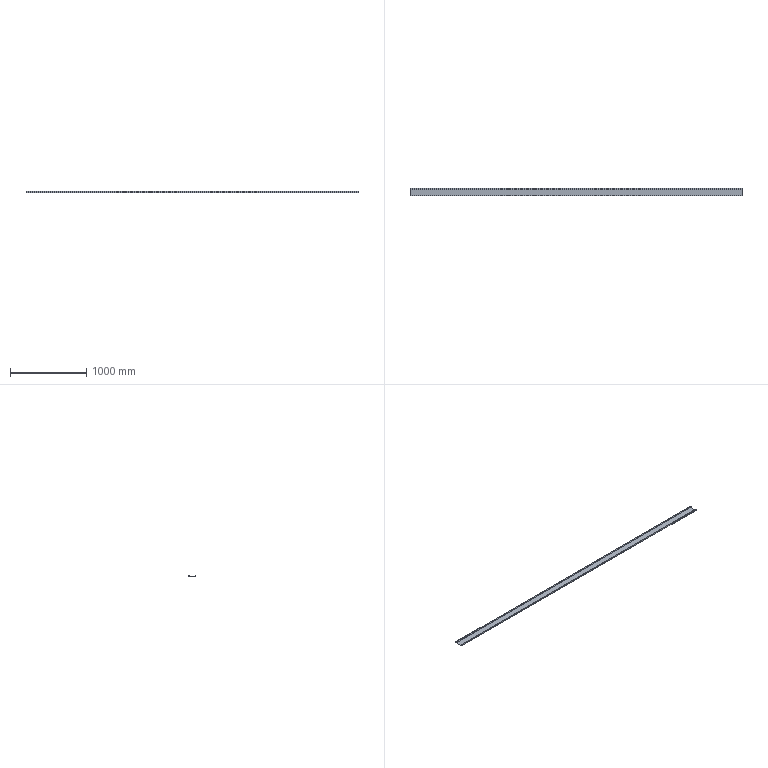Part | STEP file | 粉仓踢脚Plate 1 | 1 solid | 18 faces | box 4345 x 100 x 20 mm | volume 998785 mm3 | plane 12 | cylinder 6 | commonest cylinder face diameters 2 x3 5 x3
STEP:
#1=CARTESIAN_POINT('',(0.,0.,0.));
#2=DIRECTION('',(0.,0.,1.));
#3=DIRECTION('',(1.,0.,0.));
#4=AXIS2_PLACEMENT_3D('',#1,#2,#3);
#5=CARTESIAN_POINT('',(-2172.5,1.5,2.5));
#6=VERTEX_POINT('',#5);
#7=CARTESIAN_POINT('',(-2172.5,1.5,20.));
#8=VERTEX_POINT('',#7);
#9=CARTESIAN_POINT('',(-2172.5,1.5,2.5));
#10=DIRECTION('',(0.,0.,1.));
#11=VECTOR('',#10,1.);
#12=LINE('',#9,#11);
#13=CARTESIAN_POINT('',(2172.5,1.5,2.5));
#14=DIRECTION('',(0.,-1.,0.));
#15=DIRECTION('',(0.,0.,-1.));
#16=AXIS2_PLACEMENT_3D('',#13,#14,#15);
#17=PLANE('',#16);
#18=CARTESIAN_POINT('',(0.,-4345.));
#19=DIRECTION('',(-1.,0.));
#20=VECTOR('',#19,1.);
#21=LINE('',#18,#20);
#22=(GEOMETRIC_REPRESENTATION_CONTEXT(2)PARAMETRIC_REPRESENTATION_CONTEXT()REPRESENTATION_CONTEXT('',''));
#23=DEFINITIONAL_REPRESENTATION('',(#21),#22);
#24=PCURVE('',#17,#23);
#25=CARTESIAN_POINT('',(-2172.5,2.5,2.5));
#26=DIRECTION('',(-1.,0.,0.));
#27=DIRECTION('',(0.,0.,1.));
#28=AXIS2_PLACEMENT_3D('',#25,#26,#27);
#29=PLANE('',#28);
#30=CARTESIAN_POINT('',(0.,-1.));
#31=DIRECTION('',(1.,0.));
#32=VECTOR('',#31,1.);
#33=LINE('',#30,#32);
#34=(GEOMETRIC_REPRESENTATION_CONTEXT(2)PARAMETRIC_REPRESENTATION_CONTEXT()REPRESENTATION_CONTEXT('',''));
#35=DEFINITIONAL_REPRESENTATION('',(#33),#34);
#36=PCURVE('',#29,#35);
#37=SURFACE_CURVE('',#12,(#24,#36),.PCURVE_S1.);
#38=EDGE_CURVE('',#6,#8,#37,.T.);
#39=ORIENTED_EDGE('',*,*,#38,.T.);
#40=CARTESIAN_POINT('',(2172.5,1.5,20.));
#41=VERTEX_POINT('',#40);
#42=CARTESIAN_POINT('',(2172.5,1.5,20.));
#43=DIRECTION('',(-1.,0.,0.));
#44=VECTOR('',#43,1.);
#45=LINE('',#42,#44);
#46=CARTESIAN_POINT('',(-17.5,0.));
#47=DIRECTION('',(0.,-1.));
#48=VECTOR('',#47,1.);
#49=LINE('',#46,#48);
#50=(GEOMETRIC_REPRESENTATION_CONTEXT(2)PARAMETRIC_REPRESENTATION_CONTEXT()REPRESENTATION_CONTEXT('',''));
#51=DEFINITIONAL_REPRESENTATION('',(#49),#50);
#52=PCURVE('',#17,#51);
#53=CARTESIAN_POINT('',(2172.5,0.,20.));
#54=DIRECTION('',(0.,0.,1.));
#55=DIRECTION('',(1.,0.,0.));
#56=AXIS2_PLACEMENT_3D('',#53,#54,#55);
#57=PLANE('',#56);
#58=CARTESIAN_POINT('',(0.,1.5));
#59=DIRECTION('',(-1.,0.));
#60=VECTOR('',#59,1.);
#61=LINE('',#58,#60);
#62=(GEOMETRIC_REPRESENTATION_CONTEXT(2)PARAMETRIC_REPRESENTATION_CONTEXT()REPRESENTATION_CONTEXT('',''));
#63=DEFINITIONAL_REPRESENTATION('',(#61),#62);
#64=PCURVE('',#57,#63);
#65=SURFACE_CURVE('',#45,(#52,#64),.PCURVE_S1.);
#66=EDGE_CURVE('',#41,#8,#65,.T.);
#67=ORIENTED_EDGE('',*,*,#66,.F.);
#68=CARTESIAN_POINT('',(2172.5,1.5,2.5));
#69=VERTEX_POINT('',#68);
#70=CARTESIAN_POINT('',(2172.5,1.5,2.5));
#71=DIRECTION('',(0.,0.,1.));
#72=VECTOR('',#71,1.);
#73=LINE('',#70,#72);
#74=CARTESIAN_POINT('',(0.,0.));
#75=DIRECTION('',(-1.,0.));
#76=VECTOR('',#75,1.);
#77=LINE('',#74,#76);
#78=(GEOMETRIC_REPRESENTATION_CONTEXT(2)PARAMETRIC_REPRESENTATION_CONTEXT()REPRESENTATION_CONTEXT('',''));
#79=DEFINITIONAL_REPRESENTATION('',(#77),#78);
#80=PCURVE('',#17,#79);
#81=CARTESIAN_POINT('',(2172.5,2.5,2.5));
#82=DIRECTION('',(-1.,0.,0.));
#83=DIRECTION('',(0.,0.,1.));
#84=AXIS2_PLACEMENT_3D('',#81,#82,#83);
#85=PLANE('',#84);
#86=CARTESIAN_POINT('',(0.,-1.));
#87=DIRECTION('',(1.,0.));
#88=VECTOR('',#87,1.);
#89=LINE('',#86,#88);
#90=(GEOMETRIC_REPRESENTATION_CONTEXT(2)PARAMETRIC_REPRESENTATION_CONTEXT()REPRESENTATION_CONTEXT('',''));
#91=DEFINITIONAL_REPRESENTATION('',(#89),#90);
#92=PCURVE('',#85,#91);
#93=SURFACE_CURVE('',#73,(#80,#92),.PCURVE_S1.);
#94=EDGE_CURVE('',#69,#41,#93,.T.);
#95=ORIENTED_EDGE('',*,*,#94,.F.);
#96=CARTESIAN_POINT('',(2172.5,1.5,2.5));
#97=DIRECTION('',(-1.,0.,0.));
#98=VECTOR('',#97,1.);
#99=LINE('',#96,#98);
#100=CARTESIAN_POINT('',(0.,0.));
#101=DIRECTION('',(0.,-1.));
#102=VECTOR('',#101,1.);
#103=LINE('',#100,#102);
#104=(GEOMETRIC_REPRESENTATION_CONTEXT(2)PARAMETRIC_REPRESENTATION_CONTEXT()REPRESENTATION_CONTEXT('',''));
#105=DEFINITIONAL_REPRESENTATION('',(#103),#104);
#106=PCURVE('',#17,#105);
#107=CARTESIAN_POINT('',(2172.5,2.5,2.5));
#108=DIRECTION('',(-1.,0.,0.));
#109=DIRECTION('',(0.,0.,1.));
#110=AXIS2_PLACEMENT_3D('',#107,#108,#109);
#111=CYLINDRICAL_SURFACE('',#110,1.);
#112=CARTESIAN_POINT('',(4.712,0.));
#113=DIRECTION('',(0.,1.));
#114=VECTOR('',#113,1.);
#115=LINE('',#112,#114);
#116=(GEOMETRIC_REPRESENTATION_CONTEXT(2)PARAMETRIC_REPRESENTATION_CONTEXT()REPRESENTATION_CONTEXT('',''));
#117=DEFINITIONAL_REPRESENTATION('',(#115),#116);
#118=PCURVE('',#111,#117);
#119=SURFACE_CURVE('',#99,(#106,#118),.PCURVE_S1.);
#120=EDGE_CURVE('',#69,#6,#119,.T.);
#121=ORIENTED_EDGE('',*,*,#120,.T.);
#122=EDGE_LOOP('',(#39,#67,#95,#121));
#123=FACE_BOUND('',#122,.T.);
#124=ADVANCED_FACE('',(#123),#17,.F.);
#125=CARTESIAN_POINT('',(-2172.5,0.,20.));
#126=VERTEX_POINT('',#125);
#127=CARTESIAN_POINT('',(-2172.5,0.,20.));
#128=DIRECTION('',(0.,1.,0.));
#129=VECTOR('',#128,1.);
#130=LINE('',#127,#129);
#131=CARTESIAN_POINT('',(-4345.,0.));
#132=DIRECTION('',(0.,1.));
#133=VECTOR('',#132,1.);
#134=LINE('',#131,#133);
#135=(GEOMETRIC_REPRESENTATION_CONTEXT(2)PARAMETRIC_REPRESENTATION_CONTEXT()REPRESENTATION_CONTEXT('',''));
#136=DEFINITIONAL_REPRESENTATION('',(#134),#135);
#137=PCURVE('',#57,#136);
#138=CARTESIAN_POINT('',(17.5,-2.5));
#139=DIRECTION('',(0.,1.));
#140=VECTOR('',#139,1.);
#141=LINE('',#138,#140);
#142=(GEOMETRIC_REPRESENTATION_CONTEXT(2)PARAMETRIC_REPRESENTATION_CONTEXT()REPRESENTATION_CONTEXT('',''));
#143=DEFINITIONAL_REPRESENTATION('',(#141),#142);
#144=PCURVE('',#29,#143);
#145=SURFACE_CURVE('',#130,(#137,#144),.PCURVE_S1.);
#146=EDGE_CURVE('',#126,#8,#145,.T.);
#147=ORIENTED_EDGE('',*,*,#146,.F.);
#148=CARTESIAN_POINT('',(2172.5,0.,20.));
#149=VERTEX_POINT('',#148);
#150=CARTESIAN_POINT('',(2172.5,0.,20.));
#151=DIRECTION('',(-1.,0.,0.));
#152=VECTOR('',#151,1.);
#153=LINE('',#150,#152);
#154=CARTESIAN_POINT('',(0.,0.));
#155=DIRECTION('',(-1.,0.));
#156=VECTOR('',#155,1.);
#157=LINE('',#154,#156);
#158=(GEOMETRIC_REPRESENTATION_CONTEXT(2)PARAMETRIC_REPRESENTATION_CONTEXT()REPRESENTATION_CONTEXT('',''));
#159=DEFINITIONAL_REPRESENTATION('',(#157),#158);
#160=PCURVE('',#57,#159);
#161=CARTESIAN_POINT('',(2172.5,0.,2.5));
#162=DIRECTION('',(0.,-1.,0.));
#163=DIRECTION('',(0.,0.,-1.));
#164=AXIS2_PLACEMENT_3D('',#161,#162,#163);
#165=PLANE('',#164);
#166=CARTESIAN_POINT('',(-17.5,0.));
#167=DIRECTION('',(0.,-1.));
#168=VECTOR('',#167,1.);
#169=LINE('',#166,#168);
#170=(GEOMETRIC_REPRESENTATION_CONTEXT(2)PARAMETRIC_REPRESENTATION_CONTEXT()REPRESENTATION_CONTEXT('',''));
#171=DEFINITIONAL_REPRESENTATION('',(#169),#170);
#172=PCURVE('',#165,#171);
#173=SURFACE_CURVE('',#153,(#160,#172),.PCURVE_S1.);
#174=EDGE_CURVE('',#149,#126,#173,.T.);
#175=ORIENTED_EDGE('',*,*,#174,.F.);
#176=CARTESIAN_POINT('',(2172.5,0.,20.));
#177=DIRECTION('',(0.,1.,0.));
#178=VECTOR('',#177,1.);
#179=LINE('',#176,#178);
#180=CARTESIAN_POINT('',(0.,0.));
#181=DIRECTION('',(0.,1.));
#182=VECTOR('',#181,1.);
#183=LINE('',#180,#182);
#184=(GEOMETRIC_REPRESENTATION_CONTEXT(2)PARAMETRIC_REPRESENTATION_CONTEXT()REPRESENTATION_CONTEXT('',''));
#185=DEFINITIONAL_REPRESENTATION('',(#183),#184);
#186=PCURVE('',#57,#185);
#187=CARTESIAN_POINT('',(17.5,-2.5));
#188=DIRECTION('',(0.,1.));
#189=VECTOR('',#188,1.);
#190=LINE('',#187,#189);
#191=(GEOMETRIC_REPRESENTATION_CONTEXT(2)PARAMETRIC_REPRESENTATION_CONTEXT()REPRESENTATION_CONTEXT('',''));
#192=DEFINITIONAL_REPRESENTATION('',(#190),#191);
#193=PCURVE('',#85,#192);
#194=SURFACE_CURVE('',#179,(#186,#193),.PCURVE_S1.);
#195=EDGE_CURVE('',#149,#41,#194,.T.);
#196=ORIENTED_EDGE('',*,*,#195,.T.);
#197=ORIENTED_EDGE('',*,*,#66,.T.);
#198=EDGE_LOOP('',(#147,#175,#196,#197));
#199=FACE_BOUND('',#198,.T.);
#200=ADVANCED_FACE('',(#199),#57,.T.);
#201=CARTESIAN_POINT('',(-2172.5,0.,2.5));
#202=VERTEX_POINT('',#201);
#203=CARTESIAN_POINT('',(-2172.5,0.,2.5));
#204=DIRECTION('',(0.,0.,1.));
#205=VECTOR('',#204,1.);
#206=LINE('',#203,#205);
#207=CARTESIAN_POINT('',(0.,-4345.));
#208=DIRECTION('',(-1.,0.));
#209=VECTOR('',#208,1.);
#210=LINE('',#207,#209);
#211=(GEOMETRIC_REPRESENTATION_CONTEXT(2)PARAMETRIC_REPRESENTATION_CONTEXT()REPRESENTATION_CONTEXT('',''));
#212=DEFINITIONAL_REPRESENTATION('',(#210),#211);
#213=PCURVE('',#165,#212);
#214=CARTESIAN_POINT('',(0.,-2.5));
#215=DIRECTION('',(1.,0.));
#216=VECTOR('',#215,1.);
#217=LINE('',#214,#216);
#218=(GEOMETRIC_REPRESENTATION_CONTEXT(2)PARAMETRIC_REPRESENTATION_CONTEXT()REPRESENTATION_CONTEXT('',''));
#219=DEFINITIONAL_REPRESENTATION('',(#217),#218);
#220=PCURVE('',#29,#219);
#221=SURFACE_CURVE('',#206,(#213,#220),.PCURVE_S1.);
#222=EDGE_CURVE('',#202,#126,#221,.T.);
#223=ORIENTED_EDGE('',*,*,#222,.F.);
#224=CARTESIAN_POINT('',(2172.5,0.,2.5));
#225=VERTEX_POINT('',#224);
#226=CARTESIAN_POINT('',(2172.5,0.,2.5));
#227=DIRECTION('',(-1.,0.,0.));
#228=VECTOR('',#227,1.);
#229=LINE('',#226,#228);
#230=CARTESIAN_POINT('',(0.,0.));
#231=DIRECTION('',(0.,-1.));
#232=VECTOR('',#231,1.);
#233=LINE('',#230,#232);
#234=(GEOMETRIC_REPRESENTATION_CONTEXT(2)PARAMETRIC_REPRESENTATION_CONTEXT()REPRESENTATION_CONTEXT('',''));
#235=DEFINITIONAL_REPRESENTATION('',(#233),#234);
#236=PCURVE('',#165,#235);
#237=CARTESIAN_POINT('',(2172.5,2.5,2.5));
#238=DIRECTION('',(-1.,0.,0.));
#239=DIRECTION('',(0.,0.,1.));
#240=AXIS2_PLACEMENT_3D('',#237,#238,#239);
#241=CYLINDRICAL_SURFACE('',#240,2.5);
#242=CARTESIAN_POINT('',(4.712,0.));
#243=DIRECTION('',(0.,1.));
#244=VECTOR('',#243,1.);
#245=LINE('',#242,#244);
#246=(GEOMETRIC_REPRESENTATION_CONTEXT(2)PARAMETRIC_REPRESENTATION_CONTEXT()REPRESENTATION_CONTEXT('',''));
#247=DEFINITIONAL_REPRESENTATION('',(#245),#246);
#248=PCURVE('',#241,#247);
#249=SURFACE_CURVE('',#229,(#236,#248),.PCURVE_S1.);
#250=EDGE_CURVE('',#225,#202,#249,.T.);
#251=ORIENTED_EDGE('',*,*,#250,.F.);
#252=CARTESIAN_POINT('',(2172.5,0.,2.5));
#253=DIRECTION('',(0.,0.,1.));
#254=VECTOR('',#253,1.);
#255=LINE('',#252,#254);
#256=CARTESIAN_POINT('',(0.,0.));
#257=DIRECTION('',(-1.,0.));
#258=VECTOR('',#257,1.);
#259=LINE('',#256,#258);
#260=(GEOMETRIC_REPRESENTATION_CONTEXT(2)PARAMETRIC_REPRESENTATION_CONTEXT()REPRESENTATION_CONTEXT('',''));
#261=DEFINITIONAL_REPRESENTATION('',(#259),#260);
#262=PCURVE('',#165,#261);
#263=CARTESIAN_POINT('',(0.,-2.5));
#264=DIRECTION('',(1.,0.));
#265=VECTOR('',#264,1.);
#266=LINE('',#263,#265);
#267=(GEOMETRIC_REPRESENTATION_CONTEXT(2)PARAMETRIC_REPRESENTATION_CONTEXT()REPRESENTATION_CONTEXT('',''));
#268=DEFINITIONAL_REPRESENTATION('',(#266),#267);
#269=PCURVE('',#85,#268);
#270=SURFACE_CURVE('',#255,(#262,#269),.PCURVE_S1.);
#271=EDGE_CURVE('',#225,#149,#270,.T.);
#272=ORIENTED_EDGE('',*,*,#271,.T.);
#273=ORIENTED_EDGE('',*,*,#174,.T.);
#274=EDGE_LOOP('',(#223,#251,#272,#273));
#275=FACE_BOUND('',#274,.T.);
#276=ADVANCED_FACE('',(#275),#165,.T.);
#277=CARTESIAN_POINT('',(-2172.5,2.5,0.));
#278=VERTEX_POINT('',#277);
#279=CARTESIAN_POINT('',(-2172.5,2.5,2.5));
#280=DIRECTION('',(-1.,0.,0.));
#281=DIRECTION('',(0.,0.,1.));
#282=AXIS2_PLACEMENT_3D('',#279,#280,#281);
#283=CIRCLE('',#282,2.5);
#284=CARTESIAN_POINT('',(0.,4345.));
#285=DIRECTION('',(1.,0.));
#286=VECTOR('',#285,1.);
#287=LINE('',#284,#286);
#288=(GEOMETRIC_REPRESENTATION_CONTEXT(2)PARAMETRIC_REPRESENTATION_CONTEXT()REPRESENTATION_CONTEXT('',''));
#289=DEFINITIONAL_REPRESENTATION('',(#287),#288);
#290=PCURVE('',#241,#289);
#291=CARTESIAN_POINT('',(0.,0.));
#292=DIRECTION('',(1.,0.));
#293=AXIS2_PLACEMENT_2D('',#291,#292);
#294=CIRCLE('',#293,2.5);
#295=(GEOMETRIC_REPRESENTATION_CONTEXT(2)PARAMETRIC_REPRESENTATION_CONTEXT()REPRESENTATION_CONTEXT('',''));
#296=DEFINITIONAL_REPRESENTATION('',(#294),#295);
#297=PCURVE('',#29,#296);
#298=SURFACE_CURVE('',#283,(#290,#297),.PCURVE_S1.);
#299=EDGE_CURVE('',#278,#202,#298,.T.);
#300=ORIENTED_EDGE('',*,*,#299,.F.);
#301=CARTESIAN_POINT('',(2172.5,2.5,0.));
#302=VERTEX_POINT('',#301);
#303=CARTESIAN_POINT('',(2172.5,2.5,0.));
#304=DIRECTION('',(-1.,0.,0.));
#305=VECTOR('',#304,1.);
#306=LINE('',#303,#305);
#307=CARTESIAN_POINT('',(3.142,0.));
#308=DIRECTION('',(0.,1.));
#309=VECTOR('',#308,1.);
#310=LINE('',#307,#309);
#311=(GEOMETRIC_REPRESENTATION_CONTEXT(2)PARAMETRIC_REPRESENTATION_CONTEXT()REPRESENTATION_CONTEXT('',''));
#312=DEFINITIONAL_REPRESENTATION('',(#310),#311);
#313=PCURVE('',#241,#312);
#314=CARTESIAN_POINT('',(2172.5,2.5,0.));
#315=DIRECTION('',(0.,0.,-1.));
#316=DIRECTION('',(-1.,0.,0.));
#317=AXIS2_PLACEMENT_3D('',#314,#315,#316);
#318=PLANE('',#317);
#319=CARTESIAN_POINT('',(0.,0.));
#320=DIRECTION('',(1.,0.));
#321=VECTOR('',#320,1.);
#322=LINE('',#319,#321);
#323=(GEOMETRIC_REPRESENTATION_CONTEXT(2)PARAMETRIC_REPRESENTATION_CONTEXT()REPRESENTATION_CONTEXT('',''));
#324=DEFINITIONAL_REPRESENTATION('',(#322),#323);
#325=PCURVE('',#318,#324);
#326=SURFACE_CURVE('',#306,(#313,#325),.PCURVE_S1.);
#327=EDGE_CURVE('',#302,#278,#326,.T.);
#328=ORIENTED_EDGE('',*,*,#327,.F.);
#329=CARTESIAN_POINT('',(2172.5,2.5,2.5));
#330=DIRECTION('',(-1.,0.,0.));
#331=DIRECTION('',(0.,0.,1.));
#332=AXIS2_PLACEMENT_3D('',#329,#330,#331);
#333=CIRCLE('',#332,2.5);
#334=CARTESIAN_POINT('',(0.,0.));
#335=DIRECTION('',(1.,0.));
#336=VECTOR('',#335,1.);
#337=LINE('',#334,#336);
#338=(GEOMETRIC_REPRESENTATION_CONTEXT(2)PARAMETRIC_REPRESENTATION_CONTEXT()REPRESENTATION_CONTEXT('',''));
#339=DEFINITIONAL_REPRESENTATION('',(#337),#338);
#340=PCURVE('',#241,#339);
#341=CARTESIAN_POINT('',(0.,0.));
#342=DIRECTION('',(1.,0.));
#343=AXIS2_PLACEMENT_2D('',#341,#342);
#344=CIRCLE('',#343,2.5);
#345=(GEOMETRIC_REPRESENTATION_CONTEXT(2)PARAMETRIC_REPRESENTATION_CONTEXT()REPRESENTATION_CONTEXT('',''));
#346=DEFINITIONAL_REPRESENTATION('',(#344),#345);
#347=PCURVE('',#85,#346);
#348=SURFACE_CURVE('',#333,(#340,#347),.PCURVE_S1.);
#349=EDGE_CURVE('',#302,#225,#348,.T.);
#350=ORIENTED_EDGE('',*,*,#349,.T.);
#351=ORIENTED_EDGE('',*,*,#250,.T.);
#352=EDGE_LOOP('',(#300,#328,#350,#351));
#353=FACE_BOUND('',#352,.T.);
#354=ADVANCED_FACE('',(#353),#241,.T.);
#355=CARTESIAN_POINT('',(-2172.5,97.5,0.));
#356=VERTEX_POINT('',#355);
#357=CARTESIAN_POINT('',(-2172.5,2.5,0.));
#358=DIRECTION('',(0.,-1.,0.));
#359=VECTOR('',#358,1.);
#360=LINE('',#357,#359);
#361=CARTESIAN_POINT('',(4345.,0.));
#362=DIRECTION('',(0.,-1.));
#363=VECTOR('',#362,1.);
#364=LINE('',#361,#363);
#365=(GEOMETRIC_REPRESENTATION_CONTEXT(2)PARAMETRIC_REPRESENTATION_CONTEXT()REPRESENTATION_CONTEXT('',''));
#366=DEFINITIONAL_REPRESENTATION('',(#364),#365);
#367=PCURVE('',#318,#366);
#368=CARTESIAN_POINT('',(-2.5,0.));
#369=DIRECTION('',(0.,-1.));
#370=VECTOR('',#369,1.);
#371=LINE('',#368,#370);
#372=(GEOMETRIC_REPRESENTATION_CONTEXT(2)PARAMETRIC_REPRESENTATION_CONTEXT()REPRESENTATION_CONTEXT('',''));
#373=DEFINITIONAL_REPRESENTATION('',(#371),#372);
#374=PCURVE('',#29,#373);
#375=SURFACE_CURVE('',#360,(#367,#374),.PCURVE_S1.);
#376=EDGE_CURVE('',#356,#278,#375,.T.);
#377=ORIENTED_EDGE('',*,*,#376,.F.);
#378=CARTESIAN_POINT('',(2172.5,97.5,0.));
#379=VERTEX_POINT('',#378);
#380=CARTESIAN_POINT('',(2172.5,97.5,0.));
#381=DIRECTION('',(-1.,0.,0.));
#382=VECTOR('',#381,1.);
#383=LINE('',#380,#382);
#384=CARTESIAN_POINT('',(0.,95.));
#385=DIRECTION('',(1.,0.));
#386=VECTOR('',#385,1.);
#387=LINE('',#384,#386);
#388=(GEOMETRIC_REPRESENTATION_CONTEXT(2)PARAMETRIC_REPRESENTATION_CONTEXT()REPRESENTATION_CONTEXT('',''));
#389=DEFINITIONAL_REPRESENTATION('',(#387),#388);
#390=PCURVE('',#318,#389);
#391=CARTESIAN_POINT('',(2172.5,97.5,2.5));
#392=DIRECTION('',(-1.,0.,0.));
#393=DIRECTION('',(0.,0.,1.));
#394=AXIS2_PLACEMENT_3D('',#391,#392,#393);
#395=CYLINDRICAL_SURFACE('',#394,2.5);
#396=CARTESIAN_POINT('',(3.142,0.));
#397=DIRECTION('',(0.,1.));
#398=VECTOR('',#397,1.);
#399=LINE('',#396,#398);
#400=(GEOMETRIC_REPRESENTATION_CONTEXT(2)PARAMETRIC_REPRESENTATION_CONTEXT()REPRESENTATION_CONTEXT('',''));
#401=DEFINITIONAL_REPRESENTATION('',(#399),#400);
#402=PCURVE('',#395,#401);
#403=SURFACE_CURVE('',#383,(#390,#402),.PCURVE_S1.);
#404=EDGE_CURVE('',#379,#356,#403,.T.);
#405=ORIENTED_EDGE('',*,*,#404,.F.);
#406=CARTESIAN_POINT('',(2172.5,2.5,0.));
#407=DIRECTION('',(0.,-1.,0.));
#408=VECTOR('',#407,1.);
#409=LINE('',#406,#408);
#410=CARTESIAN_POINT('',(0.,0.));
#411=DIRECTION('',(0.,-1.));
#412=VECTOR('',#411,1.);
#413=LINE('',#410,#412);
#414=(GEOMETRIC_REPRESENTATION_CONTEXT(2)PARAMETRIC_REPRESENTATION_CONTEXT()REPRESENTATION_CONTEXT('',''));
#415=DEFINITIONAL_REPRESENTATION('',(#413),#414);
#416=PCURVE('',#318,#415);
#417=CARTESIAN_POINT('',(-2.5,0.));
#418=DIRECTION('',(0.,-1.));
#419=VECTOR('',#418,1.);
#420=LINE('',#417,#419);
#421=(GEOMETRIC_REPRESENTATION_CONTEXT(2)PARAMETRIC_REPRESENTATION_CONTEXT()REPRESENTATION_CONTEXT('',''));
#422=DEFINITIONAL_REPRESENTATION('',(#420),#421);
#423=PCURVE('',#85,#422);
#424=SURFACE_CURVE('',#409,(#416,#423),.PCURVE_S1.);
#425=EDGE_CURVE('',#379,#302,#424,.T.);
#426=ORIENTED_EDGE('',*,*,#425,.T.);
#427=ORIENTED_EDGE('',*,*,#327,.T.);
#428=EDGE_LOOP('',(#377,#405,#426,#427));
#429=FACE_BOUND('',#428,.T.);
#430=ADVANCED_FACE('',(#429),#318,.T.);
#431=CARTESIAN_POINT('',(-2172.5,100.,2.5));
#432=VERTEX_POINT('',#431);
#433=CARTESIAN_POINT('',(-2172.5,97.5,2.5));
#434=DIRECTION('',(-1.,0.,0.));
#435=DIRECTION('',(0.,0.,-1.));
#436=AXIS2_PLACEMENT_3D('',#433,#434,#435);
#437=CIRCLE('',#436,2.5);
#438=CARTESIAN_POINT('',(-3.142,4345.));
#439=DIRECTION('',(1.,0.));
#440=VECTOR('',#439,1.);
#441=LINE('',#438,#440);
#442=(GEOMETRIC_REPRESENTATION_CONTEXT(2)PARAMETRIC_REPRESENTATION_CONTEXT()REPRESENTATION_CONTEXT('',''));
#443=DEFINITIONAL_REPRESENTATION('',(#441),#442);
#444=PCURVE('',#395,#443);
#445=CARTESIAN_POINT('',(0.,95.));
#446=DIRECTION('',(-1.,0.));
#447=AXIS2_PLACEMENT_2D('',#445,#446);
#448=CIRCLE('',#447,2.5);
#449=(GEOMETRIC_REPRESENTATION_CONTEXT(2)PARAMETRIC_REPRESENTATION_CONTEXT()REPRESENTATION_CONTEXT('',''));
#450=DEFINITIONAL_REPRESENTATION('',(#448),#449);
#451=PCURVE('',#29,#450);
#452=SURFACE_CURVE('',#437,(#444,#451),.PCURVE_S1.);
#453=EDGE_CURVE('',#432,#356,#452,.T.);
#454=ORIENTED_EDGE('',*,*,#453,.F.);
#455=CARTESIAN_POINT('',(2172.5,100.,2.5));
#456=VERTEX_POINT('',#455);
#457=CARTESIAN_POINT('',(2172.5,100.,2.5));
#458=DIRECTION('',(-1.,0.,0.));
#459=VECTOR('',#458,1.);
#460=LINE('',#457,#459);
#461=CARTESIAN_POINT('',(1.571,0.));
#462=DIRECTION('',(0.,1.));
#463=VECTOR('',#462,1.);
#464=LINE('',#461,#463);
#465=(GEOMETRIC_REPRESENTATION_CONTEXT(2)PARAMETRIC_REPRESENTATION_CONTEXT()REPRESENTATION_CONTEXT('',''));
#466=DEFINITIONAL_REPRESENTATION('',(#464),#465);
#467=PCURVE('',#395,#466);
#468=CARTESIAN_POINT('',(2172.5,100.,2.5));
#469=DIRECTION('',(0.,1.,0.));
#470=DIRECTION('',(0.,0.,1.));
#471=AXIS2_PLACEMENT_3D('',#468,#469,#470);
#472=PLANE('',#471);
#473=CARTESIAN_POINT('',(0.,0.));
#474=DIRECTION('',(0.,-1.));
#475=VECTOR('',#474,1.);
#476=LINE('',#473,#475);
#477=(GEOMETRIC_REPRESENTATION_CONTEXT(2)PARAMETRIC_REPRESENTATION_CONTEXT()REPRESENTATION_CONTEXT('',''));
#478=DEFINITIONAL_REPRESENTATION('',(#476),#477);
#479=PCURVE('',#472,#478);
#480=SURFACE_CURVE('',#460,(#467,#479),.PCURVE_S1.);
#481=EDGE_CURVE('',#456,#432,#480,.T.);
#482=ORIENTED_EDGE('',*,*,#481,.F.);
#483=CARTESIAN_POINT('',(2172.5,97.5,2.5));
#484=DIRECTION('',(-1.,0.,0.));
#485=DIRECTION('',(0.,0.,-1.));
#486=AXIS2_PLACEMENT_3D('',#483,#484,#485);
#487=CIRCLE('',#486,2.5);
#488=CARTESIAN_POINT('',(-3.142,0.));
#489=DIRECTION('',(1.,0.));
#490=VECTOR('',#489,1.);
#491=LINE('',#488,#490);
#492=(GEOMETRIC_REPRESENTATION_CONTEXT(2)PARAMETRIC_REPRESENTATION_CONTEXT()REPRESENTATION_CONTEXT('',''));
#493=DEFINITIONAL_REPRESENTATION('',(#491),#492);
#494=PCURVE('',#395,#493);
#495=CARTESIAN_POINT('',(0.,95.));
#496=DIRECTION('',(-1.,0.));
#497=AXIS2_PLACEMENT_2D('',#495,#496);
#498=CIRCLE('',#497,2.5);
#499=(GEOMETRIC_REPRESENTATION_CONTEXT(2)PARAMETRIC_REPRESENTATION_CONTEXT()REPRESENTATION_CONTEXT('',''));
#500=DEFINITIONAL_REPRESENTATION('',(#498),#499);
#501=PCURVE('',#85,#500);
#502=SURFACE_CURVE('',#487,(#494,#501),.PCURVE_S1.);
#503=EDGE_CURVE('',#456,#379,#502,.T.);
#504=ORIENTED_EDGE('',*,*,#503,.T.);
#505=ORIENTED_EDGE('',*,*,#404,.T.);
#506=EDGE_LOOP('',(#454,#482,#504,#505));
#507=FACE_BOUND('',#506,.T.);
#508=ADVANCED_FACE('',(#507),#395,.T.);
#509=CARTESIAN_POINT('',(-2172.5,100.,17.5));
#510=VERTEX_POINT('',#509);
#511=CARTESIAN_POINT('',(-2172.5,100.,2.5));
#512=DIRECTION('',(0.,0.,-1.));
#513=VECTOR('',#512,1.);
#514=LINE('',#511,#513);
#515=CARTESIAN_POINT('',(0.,-4345.));
#516=DIRECTION('',(-1.,0.));
#517=VECTOR('',#516,1.);
#518=LINE('',#515,#517);
#519=(GEOMETRIC_REPRESENTATION_CONTEXT(2)PARAMETRIC_REPRESENTATION_CONTEXT()REPRESENTATION_CONTEXT('',''));
#520=DEFINITIONAL_REPRESENTATION('',(#518),#519);
#521=PCURVE('',#472,#520);
#522=CARTESIAN_POINT('',(0.,97.5));
#523=DIRECTION('',(-1.,0.));
#524=VECTOR('',#523,1.);
#525=LINE('',#522,#524);
#526=(GEOMETRIC_REPRESENTATION_CONTEXT(2)PARAMETRIC_REPRESENTATION_CONTEXT()REPRESENTATION_CONTEXT('',''));
#527=DEFINITIONAL_REPRESENTATION('',(#525),#526);
#528=PCURVE('',#29,#527);
#529=SURFACE_CURVE('',#514,(#521,#528),.PCURVE_S1.);
#530=EDGE_CURVE('',#510,#432,#529,.T.);
#531=ORIENTED_EDGE('',*,*,#530,.F.);
#532=CARTESIAN_POINT('',(2172.5,100.,17.5));
#533=VERTEX_POINT('',#532);
#534=CARTESIAN_POINT('',(2172.5,100.,17.5));
#535=DIRECTION('',(-1.,0.,0.));
#536=VECTOR('',#535,1.);
#537=LINE('',#534,#536);
#538=CARTESIAN_POINT('',(15.,0.));
#539=DIRECTION('',(0.,-1.));
#540=VECTOR('',#539,1.);
#541=LINE('',#538,#540);
#542=(GEOMETRIC_REPRESENTATION_CONTEXT(2)PARAMETRIC_REPRESENTATION_CONTEXT()REPRESENTATION_CONTEXT('',''));
#543=DEFINITIONAL_REPRESENTATION('',(#541),#542);
#544=PCURVE('',#472,#543);
#545=CARTESIAN_POINT('',(2172.5,97.5,17.5));
#546=DIRECTION('',(-1.,0.,0.));
#547=DIRECTION('',(0.,0.,1.));
#548=AXIS2_PLACEMENT_3D('',#545,#546,#547);
#549=CYLINDRICAL_SURFACE('',#548,2.5);
#550=CARTESIAN_POINT('',(1.571,0.));
#551=DIRECTION('',(0.,1.));
#552=VECTOR('',#551,1.);
#553=LINE('',#550,#552);
#554=(GEOMETRIC_REPRESENTATION_CONTEXT(2)PARAMETRIC_REPRESENTATION_CONTEXT()REPRESENTATION_CONTEXT('',''));
#555=DEFINITIONAL_REPRESENTATION('',(#553),#554);
#556=PCURVE('',#549,#555);
#557=SURFACE_CURVE('',#537,(#544,#556),.PCURVE_S1.);
#558=EDGE_CURVE('',#533,#510,#557,.T.);
#559=ORIENTED_EDGE('',*,*,#558,.F.);
#560=CARTESIAN_POINT('',(2172.5,100.,2.5));
#561=DIRECTION('',(0.,0.,-1.));
#562=VECTOR('',#561,1.);
#563=LINE('',#560,#562);
#564=CARTESIAN_POINT('',(0.,0.));
#565=DIRECTION('',(-1.,0.));
#566=VECTOR('',#565,1.);
#567=LINE('',#564,#566);
#568=(GEOMETRIC_REPRESENTATION_CONTEXT(2)PARAMETRIC_REPRESENTATION_CONTEXT()REPRESENTATION_CONTEXT('',''));
#569=DEFINITIONAL_REPRESENTATION('',(#567),#568);
#570=PCURVE('',#472,#569);
#571=CARTESIAN_POINT('',(0.,97.5));
#572=DIRECTION('',(-1.,0.));
#573=VECTOR('',#572,1.);
#574=LINE('',#571,#573);
#575=(GEOMETRIC_REPRESENTATION_CONTEXT(2)PARAMETRIC_REPRESENTATION_CONTEXT()REPRESENTATION_CONTEXT('',''));
#576=DEFINITIONAL_REPRESENTATION('',(#574),#575);
#577=PCURVE('',#85,#576);
#578=SURFACE_CURVE('',#563,(#570,#577),.PCURVE_S1.);
#579=EDGE_CURVE('',#533,#456,#578,.T.);
#580=ORIENTED_EDGE('',*,*,#579,.T.);
#581=ORIENTED_EDGE('',*,*,#481,.T.);
#582=EDGE_LOOP('',(#531,#559,#580,#581));
#583=FACE_BOUND('',#582,.T.);
#584=ADVANCED_FACE('',(#583),#472,.T.);
#585=CARTESIAN_POINT('',(-2172.5,97.5,20.));
#586=VERTEX_POINT('',#585);
#587=CARTESIAN_POINT('',(-2172.5,97.5,17.5));
#588=DIRECTION('',(-1.,0.,0.));
#589=DIRECTION('',(0.,0.,-1.));
#590=AXIS2_PLACEMENT_3D('',#587,#588,#589);
#591=CIRCLE('',#590,2.5);
#592=CARTESIAN_POINT('',(-3.142,4345.));
#593=DIRECTION('',(1.,0.));
#594=VECTOR('',#593,1.);
#595=LINE('',#592,#594);
#596=(GEOMETRIC_REPRESENTATION_CONTEXT(2)PARAMETRIC_REPRESENTATION_CONTEXT()REPRESENTATION_CONTEXT('',''));
#597=DEFINITIONAL_REPRESENTATION('',(#595),#596);
#598=PCURVE('',#549,#597);
#599=CARTESIAN_POINT('',(15.,95.));
#600=DIRECTION('',(-1.,0.));
#601=AXIS2_PLACEMENT_2D('',#599,#600);
#602=CIRCLE('',#601,2.5);
#603=(GEOMETRIC_REPRESENTATION_CONTEXT(2)PARAMETRIC_REPRESENTATION_CONTEXT()REPRESENTATION_CONTEXT('',''));
#604=DEFINITIONAL_REPRESENTATION('',(#602),#603);
#605=PCURVE('',#29,#604);
#606=SURFACE_CURVE('',#591,(#598,#605),.PCURVE_S1.);
#607=EDGE_CURVE('',#586,#510,#606,.T.);
#608=ORIENTED_EDGE('',*,*,#607,.F.);
#609=CARTESIAN_POINT('',(2172.5,97.5,20.));
#610=VERTEX_POINT('',#609);
#611=CARTESIAN_POINT('',(2172.5,97.5,20.));
#612=DIRECTION('',(-1.,0.,0.));
#613=VECTOR('',#612,1.);
#614=LINE('',#611,#613);
#615=CARTESIAN_POINT('',(0.,0.));
#616=DIRECTION('',(0.,1.));
#617=VECTOR('',#616,1.);
#618=LINE('',#615,#617);
#619=(GEOMETRIC_REPRESENTATION_CONTEXT(2)PARAMETRIC_REPRESENTATION_CONTEXT()REPRESENTATION_CONTEXT('',''));
#620=DEFINITIONAL_REPRESENTATION('',(#618),#619);
#621=PCURVE('',#549,#620);
#622=CARTESIAN_POINT('',(2172.5,97.5,20.));
#623=DIRECTION('',(0.,0.,1.));
#624=DIRECTION('',(1.,0.,0.));
#625=AXIS2_PLACEMENT_3D('',#622,#623,#624);
#626=PLANE('',#625);
#627=CARTESIAN_POINT('',(0.,0.));
#628=DIRECTION('',(-1.,0.));
#629=VECTOR('',#628,1.);
#630=LINE('',#627,#629);
#631=(GEOMETRIC_REPRESENTATION_CONTEXT(2)PARAMETRIC_REPRESENTATION_CONTEXT()REPRESENTATION_CONTEXT('',''));
#632=DEFINITIONAL_REPRESENTATION('',(#630),#631);
#633=PCURVE('',#626,#632);
#634=SURFACE_CURVE('',#614,(#621,#633),.PCURVE_S1.);
#635=EDGE_CURVE('',#610,#586,#634,.T.);
#636=ORIENTED_EDGE('',*,*,#635,.F.);
#637=CARTESIAN_POINT('',(2172.5,97.5,17.5));
#638=DIRECTION('',(-1.,0.,0.));
#639=DIRECTION('',(0.,0.,-1.));
#640=AXIS2_PLACEMENT_3D('',#637,#638,#639);
#641=CIRCLE('',#640,2.5);
#642=CARTESIAN_POINT('',(-3.142,0.));
#643=DIRECTION('',(1.,0.));
#644=VECTOR('',#643,1.);
#645=LINE('',#642,#644);
#646=(GEOMETRIC_REPRESENTATION_CONTEXT(2)PARAMETRIC_REPRESENTATION_CONTEXT()REPRESENTATION_CONTEXT('',''));
#647=DEFINITIONAL_REPRESENTATION('',(#645),#646);
#648=PCURVE('',#549,#647);
#649=CARTESIAN_POINT('',(15.,95.));
#650=DIRECTION('',(-1.,0.));
#651=AXIS2_PLACEMENT_2D('',#649,#650);
#652=CIRCLE('',#651,2.5);
#653=(GEOMETRIC_REPRESENTATION_CONTEXT(2)PARAMETRIC_REPRESENTATION_CONTEXT()REPRESENTATION_CONTEXT('',''));
#654=DEFINITIONAL_REPRESENTATION('',(#652),#653);
#655=PCURVE('',#85,#654);
#656=SURFACE_CURVE('',#641,(#648,#655),.PCURVE_S1.);
#657=EDGE_CURVE('',#610,#533,#656,.T.);
#658=ORIENTED_EDGE('',*,*,#657,.T.);
#659=ORIENTED_EDGE('',*,*,#558,.T.);
#660=EDGE_LOOP('',(#608,#636,#658,#659));
#661=FACE_BOUND('',#660,.T.);
#662=ADVANCED_FACE('',(#661),#549,.T.);
#663=CARTESIAN_POINT('',(-2172.5,80.,20.));
#664=VERTEX_POINT('',#663);
#665=CARTESIAN_POINT('',(-2172.5,97.5,20.));
#666=DIRECTION('',(0.,1.,0.));
#667=VECTOR('',#666,1.);
#668=LINE('',#665,#667);
#669=CARTESIAN_POINT('',(-4345.,0.));
#670=DIRECTION('',(0.,1.));
#671=VECTOR('',#670,1.);
#672=LINE('',#669,#671);
#673=(GEOMETRIC_REPRESENTATION_CONTEXT(2)PARAMETRIC_REPRESENTATION_CONTEXT()REPRESENTATION_CONTEXT('',''));
#674=DEFINITIONAL_REPRESENTATION('',(#672),#673);
#675=PCURVE('',#626,#674);
#676=CARTESIAN_POINT('',(17.5,95.));
#677=DIRECTION('',(0.,1.));
#678=VECTOR('',#677,1.);
#679=LINE('',#676,#678);
#680=(GEOMETRIC_REPRESENTATION_CONTEXT(2)PARAMETRIC_REPRESENTATION_CONTEXT()REPRESENTATION_CONTEXT('',''));
#681=DEFINITIONAL_REPRESENTATION('',(#679),#680);
#682=PCURVE('',#29,#681);
#683=SURFACE_CURVE('',#668,(#675,#682),.PCURVE_S1.);
#684=EDGE_CURVE('',#664,#586,#683,.T.);
#685=ORIENTED_EDGE('',*,*,#684,.F.);
#686=CARTESIAN_POINT('',(2172.5,80.,20.));
#687=VERTEX_POINT('',#686);
#688=CARTESIAN_POINT('',(2172.5,80.,20.));
#689=DIRECTION('',(-1.,0.,0.));
#690=VECTOR('',#689,1.);
#691=LINE('',#688,#690);
#692=CARTESIAN_POINT('',(0.,-17.5));
#693=DIRECTION('',(-1.,0.));
#694=VECTOR('',#693,1.);
#695=LINE('',#692,#694);
#696=(GEOMETRIC_REPRESENTATION_CONTEXT(2)PARAMETRIC_REPRESENTATION_CONTEXT()REPRESENTATION_CONTEXT('',''));
#697=DEFINITIONAL_REPRESENTATION('',(#695),#696);
#698=PCURVE('',#626,#697);
#699=CARTESIAN_POINT('',(2172.5,80.,18.5));
#700=DIRECTION('',(0.,-1.,0.));
#701=DIRECTION('',(0.,0.,-1.));
#702=AXIS2_PLACEMENT_3D('',#699,#700,#701);
#703=PLANE('',#702);
#704=CARTESIAN_POINT('',(-1.5,0.));
#705=DIRECTION('',(0.,-1.));
#706=VECTOR('',#705,1.);
#707=LINE('',#704,#706);
#708=(GEOMETRIC_REPRESENTATION_CONTEXT(2)PARAMETRIC_REPRESENTATION_CONTEXT()REPRESENTATION_CONTEXT('',''));
#709=DEFINITIONAL_REPRESENTATION('',(#707),#708);
#710=PCURVE('',#703,#709);
#711=SURFACE_CURVE('',#691,(#698,#710),.PCURVE_S1.);
#712=EDGE_CURVE('',#687,#664,#711,.T.);
#713=ORIENTED_EDGE('',*,*,#712,.F.);
#714=CARTESIAN_POINT('',(2172.5,97.5,20.));
#715=DIRECTION('',(0.,1.,0.));
#716=VECTOR('',#715,1.);
#717=LINE('',#714,#716);
#718=CARTESIAN_POINT('',(0.,0.));
#719=DIRECTION('',(0.,1.));
#720=VECTOR('',#719,1.);
#721=LINE('',#718,#720);
#722=(GEOMETRIC_REPRESENTATION_CONTEXT(2)PARAMETRIC_REPRESENTATION_CONTEXT()REPRESENTATION_CONTEXT('',''));
#723=DEFINITIONAL_REPRESENTATION('',(#721),#722);
#724=PCURVE('',#626,#723);
#725=CARTESIAN_POINT('',(17.5,95.));
#726=DIRECTION('',(0.,1.));
#727=VECTOR('',#726,1.);
#728=LINE('',#725,#727);
#729=(GEOMETRIC_REPRESENTATION_CONTEXT(2)PARAMETRIC_REPRESENTATION_CONTEXT()REPRESENTATION_CONTEXT('',''));
#730=DEFINITIONAL_REPRESENTATION('',(#728),#729);
#731=PCURVE('',#85,#730);
#732=SURFACE_CURVE('',#717,(#724,#731),.PCURVE_S1.);
#733=EDGE_CURVE('',#687,#610,#732,.T.);
#734=ORIENTED_EDGE('',*,*,#733,.T.);
#735=ORIENTED_EDGE('',*,*,#635,.T.);
#736=EDGE_LOOP('',(#685,#713,#734,#735));
#737=FACE_BOUND('',#736,.T.);
#738=ADVANCED_FACE('',(#737),#626,.T.);
#739=CARTESIAN_POINT('',(-2172.5,80.,18.5));
#740=VERTEX_POINT('',#739);
#741=CARTESIAN_POINT('',(-2172.5,80.,18.5));
#742=DIRECTION('',(0.,0.,1.));
#743=VECTOR('',#742,1.);
#744=LINE('',#741,#743);
#745=CARTESIAN_POINT('',(0.,-4345.));
#746=DIRECTION('',(-1.,0.));
#747=VECTOR('',#746,1.);
#748=LINE('',#745,#747);
#749=(GEOMETRIC_REPRESENTATION_CONTEXT(2)PARAMETRIC_REPRESENTATION_CONTEXT()REPRESENTATION_CONTEXT('',''));
#750=DEFINITIONAL_REPRESENTATION('',(#748),#749);
#751=PCURVE('',#703,#750);
#752=CARTESIAN_POINT('',(16.,77.5));
#753=DIRECTION('',(1.,0.));
#754=VECTOR('',#753,1.);
#755=LINE('',#752,#754);
#756=(GEOMETRIC_REPRESENTATION_CONTEXT(2)PARAMETRIC_REPRESENTATION_CONTEXT()REPRESENTATION_CONTEXT('',''));
#757=DEFINITIONAL_REPRESENTATION('',(#755),#756);
#758=PCURVE('',#29,#757);
#759=SURFACE_CURVE('',#744,(#751,#758),.PCURVE_S1.);
#760=EDGE_CURVE('',#740,#664,#759,.T.);
#761=ORIENTED_EDGE('',*,*,#760,.F.);
#762=CARTESIAN_POINT('',(2172.5,80.,18.5));
#763=VERTEX_POINT('',#762);
#764=CARTESIAN_POINT('',(2172.5,80.,18.5));
#765=DIRECTION('',(-1.,0.,0.));
#766=VECTOR('',#765,1.);
#767=LINE('',#764,#766);
#768=CARTESIAN_POINT('',(0.,0.));
#769=DIRECTION('',(0.,-1.));
#770=VECTOR('',#769,1.);
#771=LINE('',#768,#770);
#772=(GEOMETRIC_REPRESENTATION_CONTEXT(2)PARAMETRIC_REPRESENTATION_CONTEXT()REPRESENTATION_CONTEXT('',''));
#773=DEFINITIONAL_REPRESENTATION('',(#771),#772);
#774=PCURVE('',#703,#773);
#775=CARTESIAN_POINT('',(2172.5,97.5,18.5));
#776=DIRECTION('',(0.,0.,1.));
#777=DIRECTION('',(1.,0.,0.));
#778=AXIS2_PLACEMENT_3D('',#775,#776,#777);
#779=PLANE('',#778);
#780=CARTESIAN_POINT('',(0.,-17.5));
#781=DIRECTION('',(-1.,0.));
#782=VECTOR('',#781,1.);
#783=LINE('',#780,#782);
#784=(GEOMETRIC_REPRESENTATION_CONTEXT(2)PARAMETRIC_REPRESENTATION_CONTEXT()REPRESENTATION_CONTEXT('',''));
#785=DEFINITIONAL_REPRESENTATION('',(#783),#784);
#786=PCURVE('',#779,#785);
#787=SURFACE_CURVE('',#767,(#774,#786),.PCURVE_S1.);
#788=EDGE_CURVE('',#763,#740,#787,.T.);
#789=ORIENTED_EDGE('',*,*,#788,.F.);
#790=CARTESIAN_POINT('',(2172.5,80.,18.5));
#791=DIRECTION('',(0.,0.,1.));
#792=VECTOR('',#791,1.);
#793=LINE('',#790,#792);
#794=CARTESIAN_POINT('',(0.,0.));
#795=DIRECTION('',(-1.,0.));
#796=VECTOR('',#795,1.);
#797=LINE('',#794,#796);
#798=(GEOMETRIC_REPRESENTATION_CONTEXT(2)PARAMETRIC_REPRESENTATION_CONTEXT()REPRESENTATION_CONTEXT('',''));
#799=DEFINITIONAL_REPRESENTATION('',(#797),#798);
#800=PCURVE('',#703,#799);
#801=CARTESIAN_POINT('',(16.,77.5));
#802=DIRECTION('',(1.,0.));
#803=VECTOR('',#802,1.);
#804=LINE('',#801,#803);
#805=(GEOMETRIC_REPRESENTATION_CONTEXT(2)PARAMETRIC_REPRESENTATION_CONTEXT()REPRESENTATION_CONTEXT('',''));
#806=DEFINITIONAL_REPRESENTATION('',(#804),#805);
#807=PCURVE('',#85,#806);
#808=SURFACE_CURVE('',#793,(#800,#807),.PCURVE_S1.);
#809=EDGE_CURVE('',#763,#687,#808,.T.);
#810=ORIENTED_EDGE('',*,*,#809,.T.);
#811=ORIENTED_EDGE('',*,*,#712,.T.);
#812=EDGE_LOOP('',(#761,#789,#810,#811));
#813=FACE_BOUND('',#812,.T.);
#814=ADVANCED_FACE('',(#813),#703,.T.);
#815=CARTESIAN_POINT('',(-2172.5,97.5,18.5));
#816=VERTEX_POINT('',#815);
#817=CARTESIAN_POINT('',(-2172.5,97.5,18.5));
#818=DIRECTION('',(0.,1.,0.));
#819=VECTOR('',#818,1.);
#820=LINE('',#817,#819);
#821=CARTESIAN_POINT('',(-4345.,0.));
#822=DIRECTION('',(0.,1.));
#823=VECTOR('',#822,1.);
#824=LINE('',#821,#823);
#825=(GEOMETRIC_REPRESENTATION_CONTEXT(2)PARAMETRIC_REPRESENTATION_CONTEXT()REPRESENTATION_CONTEXT('',''));
#826=DEFINITIONAL_REPRESENTATION('',(#824),#825);
#827=PCURVE('',#779,#826);
#828=CARTESIAN_POINT('',(16.,95.));
#829=DIRECTION('',(0.,1.));
#830=VECTOR('',#829,1.);
#831=LINE('',#828,#830);
#832=(GEOMETRIC_REPRESENTATION_CONTEXT(2)PARAMETRIC_REPRESENTATION_CONTEXT()REPRESENTATION_CONTEXT('',''));
#833=DEFINITIONAL_REPRESENTATION('',(#831),#832);
#834=PCURVE('',#29,#833);
#835=SURFACE_CURVE('',#820,(#827,#834),.PCURVE_S1.);
#836=EDGE_CURVE('',#740,#816,#835,.T.);
#837=ORIENTED_EDGE('',*,*,#836,.T.);
#838=CARTESIAN_POINT('',(2172.5,97.5,18.5));
#839=VERTEX_POINT('',#838);
#840=CARTESIAN_POINT('',(2172.5,97.5,18.5));
#841=DIRECTION('',(-1.,0.,0.));
#842=VECTOR('',#841,1.);
#843=LINE('',#840,#842);
#844=CARTESIAN_POINT('',(0.,0.));
#845=DIRECTION('',(-1.,0.));
#846=VECTOR('',#845,1.);
#847=LINE('',#844,#846);
#848=(GEOMETRIC_REPRESENTATION_CONTEXT(2)PARAMETRIC_REPRESENTATION_CONTEXT()REPRESENTATION_CONTEXT('',''));
#849=DEFINITIONAL_REPRESENTATION('',(#847),#848);
#850=PCURVE('',#779,#849);
#851=CARTESIAN_POINT('',(2172.5,97.5,17.5));
#852=DIRECTION('',(-1.,0.,0.));
#853=DIRECTION('',(0.,0.,1.));
#854=AXIS2_PLACEMENT_3D('',#851,#852,#853);
#855=CYLINDRICAL_SURFACE('',#854,1.);
#856=CARTESIAN_POINT('',(0.,0.));
#857=DIRECTION('',(0.,1.));
#858=VECTOR('',#857,1.);
#859=LINE('',#856,#858);
#860=(GEOMETRIC_REPRESENTATION_CONTEXT(2)PARAMETRIC_REPRESENTATION_CONTEXT()REPRESENTATION_CONTEXT('',''));
#861=DEFINITIONAL_REPRESENTATION('',(#859),#860);
#862=PCURVE('',#855,#861);
#863=SURFACE_CURVE('',#843,(#850,#862),.PCURVE_S1.);
#864=EDGE_CURVE('',#839,#816,#863,.T.);
#865=ORIENTED_EDGE('',*,*,#864,.F.);
#866=CARTESIAN_POINT('',(2172.5,97.5,18.5));
#867=DIRECTION('',(0.,1.,0.));
#868=VECTOR('',#867,1.);
#869=LINE('',#866,#868);
#870=CARTESIAN_POINT('',(0.,0.));
#871=DIRECTION('',(0.,1.));
#872=VECTOR('',#871,1.);
#873=LINE('',#870,#872);
#874=(GEOMETRIC_REPRESENTATION_CONTEXT(2)PARAMETRIC_REPRESENTATION_CONTEXT()REPRESENTATION_CONTEXT('',''));
#875=DEFINITIONAL_REPRESENTATION('',(#873),#874);
#876=PCURVE('',#779,#875);
#877=CARTESIAN_POINT('',(16.,95.));
#878=DIRECTION('',(0.,1.));
#879=VECTOR('',#878,1.);
#880=LINE('',#877,#879);
#881=(GEOMETRIC_REPRESENTATION_CONTEXT(2)PARAMETRIC_REPRESENTATION_CONTEXT()REPRESENTATION_CONTEXT('',''));
#882=DEFINITIONAL_REPRESENTATION('',(#880),#881);
#883=PCURVE('',#85,#882);
#884=SURFACE_CURVE('',#869,(#876,#883),.PCURVE_S1.);
#885=EDGE_CURVE('',#763,#839,#884,.T.);
#886=ORIENTED_EDGE('',*,*,#885,.F.);
#887=ORIENTED_EDGE('',*,*,#788,.T.);
#888=EDGE_LOOP('',(#837,#865,#886,#887));
#889=FACE_BOUND('',#888,.T.);
#890=ADVANCED_FACE('',(#889),#779,.F.);
#891=ORIENTED_EDGE('',*,*,#864,.F.);
#892=CARTESIAN_POINT('',(2172.5,98.5,17.5));
#893=VERTEX_POINT('',#892);
#894=CARTESIAN_POINT('',(2172.5,97.5,17.5));
#895=DIRECTION('',(-1.,0.,0.));
#896=DIRECTION('',(0.,0.,-1.));
#897=AXIS2_PLACEMENT_3D('',#894,#895,#896);
#898=CIRCLE('',#897,1.);
#899=CARTESIAN_POINT('',(-3.142,0.));
#900=DIRECTION('',(1.,0.));
#901=VECTOR('',#900,1.);
#902=LINE('',#899,#901);
#903=(GEOMETRIC_REPRESENTATION_CONTEXT(2)PARAMETRIC_REPRESENTATION_CONTEXT()REPRESENTATION_CONTEXT('',''));
#904=DEFINITIONAL_REPRESENTATION('',(#902),#903);
#905=PCURVE('',#855,#904);
#906=CARTESIAN_POINT('',(15.,95.));
#907=DIRECTION('',(-1.,0.));
#908=AXIS2_PLACEMENT_2D('',#906,#907);
#909=CIRCLE('',#908,1.);
#910=(GEOMETRIC_REPRESENTATION_CONTEXT(2)PARAMETRIC_REPRESENTATION_CONTEXT()REPRESENTATION_CONTEXT('',''));
#911=DEFINITIONAL_REPRESENTATION('',(#909),#910);
#912=PCURVE('',#85,#911);
#913=SURFACE_CURVE('',#898,(#905,#912),.PCURVE_S1.);
#914=EDGE_CURVE('',#839,#893,#913,.T.);
#915=ORIENTED_EDGE('',*,*,#914,.T.);
#916=CARTESIAN_POINT('',(-2172.5,98.5,17.5));
#917=VERTEX_POINT('',#916);
#918=CARTESIAN_POINT('',(2172.5,98.5,17.5));
#919=DIRECTION('',(-1.,0.,0.));
#920=VECTOR('',#919,1.);
#921=LINE('',#918,#920);
#922=CARTESIAN_POINT('',(1.571,0.));
#923=DIRECTION('',(0.,1.));
#924=VECTOR('',#923,1.);
#925=LINE('',#922,#924);
#926=(GEOMETRIC_REPRESENTATION_CONTEXT(2)PARAMETRIC_REPRESENTATION_CONTEXT()REPRESENTATION_CONTEXT('',''));
#927=DEFINITIONAL_REPRESENTATION('',(#925),#926);
#928=PCURVE('',#855,#927);
#929=CARTESIAN_POINT('',(2172.5,98.5,2.5));
#930=DIRECTION('',(0.,1.,0.));
#931=DIRECTION('',(0.,0.,1.));
#932=AXIS2_PLACEMENT_3D('',#929,#930,#931);
#933=PLANE('',#932);
#934=CARTESIAN_POINT('',(15.,0.));
#935=DIRECTION('',(0.,-1.));
#936=VECTOR('',#935,1.);
#937=LINE('',#934,#936);
#938=(GEOMETRIC_REPRESENTATION_CONTEXT(2)PARAMETRIC_REPRESENTATION_CONTEXT()REPRESENTATION_CONTEXT('',''));
#939=DEFINITIONAL_REPRESENTATION('',(#937),#938);
#940=PCURVE('',#933,#939);
#941=SURFACE_CURVE('',#921,(#928,#940),.PCURVE_S1.);
#942=EDGE_CURVE('',#893,#917,#941,.T.);
#943=ORIENTED_EDGE('',*,*,#942,.T.);
#944=CARTESIAN_POINT('',(-2172.5,97.5,17.5));
#945=DIRECTION('',(-1.,0.,0.));
#946=DIRECTION('',(0.,0.,-1.));
#947=AXIS2_PLACEMENT_3D('',#944,#945,#946);
#948=CIRCLE('',#947,1.);
#949=CARTESIAN_POINT('',(-3.142,4345.));
#950=DIRECTION('',(1.,0.));
#951=VECTOR('',#950,1.);
#952=LINE('',#949,#951);
#953=(GEOMETRIC_REPRESENTATION_CONTEXT(2)PARAMETRIC_REPRESENTATION_CONTEXT()REPRESENTATION_CONTEXT('',''));
#954=DEFINITIONAL_REPRESENTATION('',(#952),#953);
#955=PCURVE('',#855,#954);
#956=CARTESIAN_POINT('',(15.,95.));
#957=DIRECTION('',(-1.,0.));
#958=AXIS2_PLACEMENT_2D('',#956,#957);
#959=CIRCLE('',#958,1.);
#960=(GEOMETRIC_REPRESENTATION_CONTEXT(2)PARAMETRIC_REPRESENTATION_CONTEXT()REPRESENTATION_CONTEXT('',''));
#961=DEFINITIONAL_REPRESENTATION('',(#959),#960);
#962=PCURVE('',#29,#961);
#963=SURFACE_CURVE('',#948,(#955,#962),.PCURVE_S1.);
#964=EDGE_CURVE('',#816,#917,#963,.T.);
#965=ORIENTED_EDGE('',*,*,#964,.F.);
#966=EDGE_LOOP('',(#891,#915,#943,#965));
#967=FACE_BOUND('',#966,.F.);
#968=ADVANCED_FACE('',(#967),#855,.F.);
#969=CARTESIAN_POINT('',(-2172.5,98.5,2.5));
#970=VERTEX_POINT('',#969);
#971=CARTESIAN_POINT('',(-2172.5,98.5,2.5));
#972=DIRECTION('',(0.,0.,-1.));
#973=VECTOR('',#972,1.);
#974=LINE('',#971,#973);
#975=CARTESIAN_POINT('',(0.,-4345.));
#976=DIRECTION('',(-1.,0.));
#977=VECTOR('',#976,1.);
#978=LINE('',#975,#977);
#979=(GEOMETRIC_REPRESENTATION_CONTEXT(2)PARAMETRIC_REPRESENTATION_CONTEXT()REPRESENTATION_CONTEXT('',''));
#980=DEFINITIONAL_REPRESENTATION('',(#978),#979);
#981=PCURVE('',#933,#980);
#982=CARTESIAN_POINT('',(0.,96.));
#983=DIRECTION('',(-1.,0.));
#984=VECTOR('',#983,1.);
#985=LINE('',#982,#984);
#986=(GEOMETRIC_REPRESENTATION_CONTEXT(2)PARAMETRIC_REPRESENTATION_CONTEXT()REPRESENTATION_CONTEXT('',''));
#987=DEFINITIONAL_REPRESENTATION('',(#985),#986);
#988=PCURVE('',#29,#987);
#989=SURFACE_CURVE('',#974,(#981,#988),.PCURVE_S1.);
#990=EDGE_CURVE('',#917,#970,#989,.T.);
#991=ORIENTED_EDGE('',*,*,#990,.T.);
#992=CARTESIAN_POINT('',(2172.5,98.5,2.5));
#993=VERTEX_POINT('',#992);
#994=CARTESIAN_POINT('',(2172.5,98.5,2.5));
#995=DIRECTION('',(-1.,0.,0.));
#996=VECTOR('',#995,1.);
#997=LINE('',#994,#996);
#998=CARTESIAN_POINT('',(0.,0.));
#999=DIRECTION('',(0.,-1.));
#1000=VECTOR('',#999,1.);
#1001=LINE('',#998,#1000);
#1002=(GEOMETRIC_REPRESENTATION_CONTEXT(2)PARAMETRIC_REPRESENTATION_CONTEXT()REPRESENTATION_CONTEXT('',''));
#1003=DEFINITIONAL_REPRESENTATION('',(#1001),#1002);
#1004=PCURVE('',#933,#1003);
#1005=CARTESIAN_POINT('',(2172.5,97.5,2.5));
#1006=DIRECTION('',(-1.,0.,0.));
#1007=DIRECTION('',(0.,0.,1.));
#1008=AXIS2_PLACEMENT_3D('',#1005,#1006,#1007);
#1009=CYLINDRICAL_SURFACE('',#1008,1.);
#1010=CARTESIAN_POINT('',(1.571,0.));
#1011=DIRECTION('',(0.,1.));
#1012=VECTOR('',#1011,1.);
#1013=LINE('',#1010,#1012);
#1014=(GEOMETRIC_REPRESENTATION_CONTEXT(2)PARAMETRIC_REPRESENTATION_CONTEXT()REPRESENTATION_CONTEXT('',''));
#1015=DEFINITIONAL_REPRESENTATION('',(#1013),#1014);
#1016=PCURVE('',#1009,#1015);
#1017=SURFACE_CURVE('',#997,(#1004,#1016),.PCURVE_S1.);
#1018=EDGE_CURVE('',#993,#970,#1017,.T.);
#1019=ORIENTED_EDGE('',*,*,#1018,.F.);
#1020=CARTESIAN_POINT('',(2172.5,98.5,2.5));
#1021=DIRECTION('',(0.,0.,-1.));
#1022=VECTOR('',#1021,1.);
#1023=LINE('',#1020,#1022);
#1024=CARTESIAN_POINT('',(0.,0.));
#1025=DIRECTION('',(-1.,0.));
#1026=VECTOR('',#1025,1.);
#1027=LINE('',#1024,#1026);
#1028=(GEOMETRIC_REPRESENTATION_CONTEXT(2)PARAMETRIC_REPRESENTATION_CONTEXT()REPRESENTATION_CONTEXT('',''));
#1029=DEFINITIONAL_REPRESENTATION('',(#1027),#1028);
#1030=PCURVE('',#933,#1029);
#1031=CARTESIAN_POINT('',(0.,96.));
#1032=DIRECTION('',(-1.,0.));
#1033=VECTOR('',#1032,1.);
#1034=LINE('',#1031,#1033);
#1035=(GEOMETRIC_REPRESENTATION_CONTEXT(2)PARAMETRIC_REPRESENTATION_CONTEXT()REPRESENTATION_CONTEXT('',''));
#1036=DEFINITIONAL_REPRESENTATION('',(#1034),#1035);
#1037=PCURVE('',#85,#1036);
#1038=SURFACE_CURVE('',#1023,(#1030,#1037),.PCURVE_S1.);
#1039=EDGE_CURVE('',#893,#993,#1038,.T.);
#1040=ORIENTED_EDGE('',*,*,#1039,.F.);
#1041=ORIENTED_EDGE('',*,*,#942,.T.);
#1042=EDGE_LOOP('',(#991,#1019,#1040,#1041));
#1043=FACE_BOUND('',#1042,.T.);
#1044=ADVANCED_FACE('',(#1043),#933,.F.);
#1045=ORIENTED_EDGE('',*,*,#1018,.F.);
#1046=CARTESIAN_POINT('',(2172.5,97.5,1.5));
#1047=VERTEX_POINT('',#1046);
#1048=CARTESIAN_POINT('',(2172.5,97.5,2.5));
#1049=DIRECTION('',(-1.,0.,0.));
#1050=DIRECTION('',(0.,0.,-1.));
#1051=AXIS2_PLACEMENT_3D('',#1048,#1049,#1050);
#1052=CIRCLE('',#1051,1.);
#1053=CARTESIAN_POINT('',(-3.142,0.));
#1054=DIRECTION('',(1.,0.));
#1055=VECTOR('',#1054,1.);
#1056=LINE('',#1053,#1055);
#1057=(GEOMETRIC_REPRESENTATION_CONTEXT(2)PARAMETRIC_REPRESENTATION_CONTEXT()REPRESENTATION_CONTEXT('',''));
#1058=DEFINITIONAL_REPRESENTATION('',(#1056),#1057);
#1059=PCURVE('',#1009,#1058);
#1060=CARTESIAN_POINT('',(0.,95.));
#1061=DIRECTION('',(-1.,0.));
#1062=AXIS2_PLACEMENT_2D('',#1060,#1061);
#1063=CIRCLE('',#1062,1.);
#1064=(GEOMETRIC_REPRESENTATION_CONTEXT(2)PARAMETRIC_REPRESENTATION_CONTEXT()REPRESENTATION_CONTEXT('',''));
#1065=DEFINITIONAL_REPRESENTATION('',(#1063),#1064);
#1066=PCURVE('',#85,#1065);
#1067=SURFACE_CURVE('',#1052,(#1059,#1066),.PCURVE_S1.);
#1068=EDGE_CURVE('',#993,#1047,#1067,.T.);
#1069=ORIENTED_EDGE('',*,*,#1068,.T.);
#1070=CARTESIAN_POINT('',(-2172.5,97.5,1.5));
#1071=VERTEX_POINT('',#1070);
#1072=CARTESIAN_POINT('',(2172.5,97.5,1.5));
#1073=DIRECTION('',(-1.,0.,0.));
#1074=VECTOR('',#1073,1.);
#1075=LINE('',#1072,#1074);
#1076=CARTESIAN_POINT('',(3.142,0.));
#1077=DIRECTION('',(0.,1.));
#1078=VECTOR('',#1077,1.);
#1079=LINE('',#1076,#1078);
#1080=(GEOMETRIC_REPRESENTATION_CONTEXT(2)PARAMETRIC_REPRESENTATION_CONTEXT()REPRESENTATION_CONTEXT('',''));
#1081=DEFINITIONAL_REPRESENTATION('',(#1079),#1080);
#1082=PCURVE('',#1009,#1081);
#1083=CARTESIAN_POINT('',(2172.5,2.5,1.5));
#1084=DIRECTION('',(0.,0.,-1.));
#1085=DIRECTION('',(-1.,0.,0.));
#1086=AXIS2_PLACEMENT_3D('',#1083,#1084,#1085);
#1087=PLANE('',#1086);
#1088=CARTESIAN_POINT('',(0.,95.));
#1089=DIRECTION('',(1.,0.));
#1090=VECTOR('',#1089,1.);
#1091=LINE('',#1088,#1090);
#1092=(GEOMETRIC_REPRESENTATION_CONTEXT(2)PARAMETRIC_REPRESENTATION_CONTEXT()REPRESENTATION_CONTEXT('',''));
#1093=DEFINITIONAL_REPRESENTATION('',(#1091),#1092);
#1094=PCURVE('',#1087,#1093);
#1095=SURFACE_CURVE('',#1075,(#1082,#1094),.PCURVE_S1.);
#1096=EDGE_CURVE('',#1047,#1071,#1095,.T.);
#1097=ORIENTED_EDGE('',*,*,#1096,.T.);
#1098=CARTESIAN_POINT('',(-2172.5,97.5,2.5));
#1099=DIRECTION('',(-1.,0.,0.));
#1100=DIRECTION('',(0.,0.,-1.));
#1101=AXIS2_PLACEMENT_3D('',#1098,#1099,#1100);
#1102=CIRCLE('',#1101,1.);
#1103=CARTESIAN_POINT('',(-3.142,4345.));
#1104=DIRECTION('',(1.,0.));
#1105=VECTOR('',#1104,1.);
#1106=LINE('',#1103,#1105);
#1107=(GEOMETRIC_REPRESENTATION_CONTEXT(2)PARAMETRIC_REPRESENTATION_CONTEXT()REPRESENTATION_CONTEXT('',''));
#1108=DEFINITIONAL_REPRESENTATION('',(#1106),#1107);
#1109=PCURVE('',#1009,#1108);
#1110=CARTESIAN_POINT('',(0.,95.));
#1111=DIRECTION('',(-1.,0.));
#1112=AXIS2_PLACEMENT_2D('',#1110,#1111);
#1113=CIRCLE('',#1112,1.);
#1114=(GEOMETRIC_REPRESENTATION_CONTEXT(2)PARAMETRIC_REPRESENTATION_CONTEXT()REPRESENTATION_CONTEXT('',''));
#1115=DEFINITIONAL_REPRESENTATION('',(#1113),#1114);
#1116=PCURVE('',#29,#1115);
#1117=SURFACE_CURVE('',#1102,(#1109,#1116),.PCURVE_S1.);
#1118=EDGE_CURVE('',#970,#1071,#1117,.T.);
#1119=ORIENTED_EDGE('',*,*,#1118,.F.);
#1120=EDGE_LOOP('',(#1045,#1069,#1097,#1119));
#1121=FACE_BOUND('',#1120,.F.);
#1122=ADVANCED_FACE('',(#1121),#1009,.F.);
#1123=CARTESIAN_POINT('',(-2172.5,2.5,1.5));
#1124=VERTEX_POINT('',#1123);
#1125=CARTESIAN_POINT('',(-2172.5,2.5,1.5));
#1126=DIRECTION('',(0.,-1.,0.));
#1127=VECTOR('',#1126,1.);
#1128=LINE('',#1125,#1127);
#1129=CARTESIAN_POINT('',(4345.,0.));
#1130=DIRECTION('',(0.,-1.));
#1131=VECTOR('',#1130,1.);
#1132=LINE('',#1129,#1131);
#1133=(GEOMETRIC_REPRESENTATION_CONTEXT(2)PARAMETRIC_REPRESENTATION_CONTEXT()REPRESENTATION_CONTEXT('',''));
#1134=DEFINITIONAL_REPRESENTATION('',(#1132),#1133);
#1135=PCURVE('',#1087,#1134);
#1136=CARTESIAN_POINT('',(-1.,0.));
#1137=DIRECTION('',(0.,-1.));
#1138=VECTOR('',#1137,1.);
#1139=LINE('',#1136,#1138);
#1140=(GEOMETRIC_REPRESENTATION_CONTEXT(2)PARAMETRIC_REPRESENTATION_CONTEXT()REPRESENTATION_CONTEXT('',''));
#1141=DEFINITIONAL_REPRESENTATION('',(#1139),#1140);
#1142=PCURVE('',#29,#1141);
#1143=SURFACE_CURVE('',#1128,(#1135,#1142),.PCURVE_S1.);
#1144=EDGE_CURVE('',#1071,#1124,#1143,.T.);
#1145=ORIENTED_EDGE('',*,*,#1144,.T.);
#1146=CARTESIAN_POINT('',(2172.5,2.5,1.5));
#1147=VERTEX_POINT('',#1146);
#1148=CARTESIAN_POINT('',(2172.5,2.5,1.5));
#1149=DIRECTION('',(-1.,0.,0.));
#1150=VECTOR('',#1149,1.);
#1151=LINE('',#1148,#1150);
#1152=CARTESIAN_POINT('',(0.,0.));
#1153=DIRECTION('',(1.,0.));
#1154=VECTOR('',#1153,1.);
#1155=LINE('',#1152,#1154);
#1156=(GEOMETRIC_REPRESENTATION_CONTEXT(2)PARAMETRIC_REPRESENTATION_CONTEXT()REPRESENTATION_CONTEXT('',''));
#1157=DEFINITIONAL_REPRESENTATION('',(#1155),#1156);
#1158=PCURVE('',#1087,#1157);
#1159=CARTESIAN_POINT('',(3.142,0.));
#1160=DIRECTION('',(0.,1.));
#1161=VECTOR('',#1160,1.);
#1162=LINE('',#1159,#1161);
#1163=(GEOMETRIC_REPRESENTATION_CONTEXT(2)PARAMETRIC_REPRESENTATION_CONTEXT()REPRESENTATION_CONTEXT('',''));
#1164=DEFINITIONAL_REPRESENTATION('',(#1162),#1163);
#1165=PCURVE('',#111,#1164);
#1166=SURFACE_CURVE('',#1151,(#1158,#1165),.PCURVE_S1.);
#1167=EDGE_CURVE('',#1147,#1124,#1166,.T.);
#1168=ORIENTED_EDGE('',*,*,#1167,.F.);
#1169=CARTESIAN_POINT('',(2172.5,2.5,1.5));
#1170=DIRECTION('',(0.,-1.,0.));
#1171=VECTOR('',#1170,1.);
#1172=LINE('',#1169,#1171);
#1173=CARTESIAN_POINT('',(0.,0.));
#1174=DIRECTION('',(0.,-1.));
#1175=VECTOR('',#1174,1.);
#1176=LINE('',#1173,#1175);
#1177=(GEOMETRIC_REPRESENTATION_CONTEXT(2)PARAMETRIC_REPRESENTATION_CONTEXT()REPRESENTATION_CONTEXT('',''));
#1178=DEFINITIONAL_REPRESENTATION('',(#1176),#1177);
#1179=PCURVE('',#1087,#1178);
#1180=CARTESIAN_POINT('',(-1.,0.));
#1181=DIRECTION('',(0.,-1.));
#1182=VECTOR('',#1181,1.);
#1183=LINE('',#1180,#1182);
#1184=(GEOMETRIC_REPRESENTATION_CONTEXT(2)PARAMETRIC_REPRESENTATION_CONTEXT()REPRESENTATION_CONTEXT('',''));
#1185=DEFINITIONAL_REPRESENTATION('',(#1183),#1184);
#1186=PCURVE('',#85,#1185);
#1187=SURFACE_CURVE('',#1172,(#1179,#1186),.PCURVE_S1.);
#1188=EDGE_CURVE('',#1047,#1147,#1187,.T.);
#1189=ORIENTED_EDGE('',*,*,#1188,.F.);
#1190=ORIENTED_EDGE('',*,*,#1096,.T.);
#1191=EDGE_LOOP('',(#1145,#1168,#1189,#1190));
#1192=FACE_BOUND('',#1191,.T.);
#1193=ADVANCED_FACE('',(#1192),#1087,.F.);
#1194=ORIENTED_EDGE('',*,*,#1167,.F.);
#1195=CARTESIAN_POINT('',(2172.5,2.5,2.5));
#1196=DIRECTION('',(-1.,0.,0.));
#1197=DIRECTION('',(0.,0.,-1.));
#1198=AXIS2_PLACEMENT_3D('',#1195,#1196,#1197);
#1199=CIRCLE('',#1198,1.);
#1200=CARTESIAN_POINT('',(3.142,0.));
#1201=DIRECTION('',(1.,0.));
#1202=VECTOR('',#1201,1.);
#1203=LINE('',#1200,#1202);
#1204=(GEOMETRIC_REPRESENTATION_CONTEXT(2)PARAMETRIC_REPRESENTATION_CONTEXT()REPRESENTATION_CONTEXT('',''));
#1205=DEFINITIONAL_REPRESENTATION('',(#1203),#1204);
#1206=PCURVE('',#111,#1205);
#1207=CARTESIAN_POINT('',(0.,0.));
#1208=DIRECTION('',(-1.,0.));
#1209=AXIS2_PLACEMENT_2D('',#1207,#1208);
#1210=CIRCLE('',#1209,1.);
#1211=(GEOMETRIC_REPRESENTATION_CONTEXT(2)PARAMETRIC_REPRESENTATION_CONTEXT()REPRESENTATION_CONTEXT('',''));
#1212=DEFINITIONAL_REPRESENTATION('',(#1210),#1211);
#1213=PCURVE('',#85,#1212);
#1214=SURFACE_CURVE('',#1199,(#1206,#1213),.PCURVE_S1.);
#1215=EDGE_CURVE('',#1147,#69,#1214,.T.);
#1216=ORIENTED_EDGE('',*,*,#1215,.T.);
#1217=ORIENTED_EDGE('',*,*,#120,.T.);
#1218=CARTESIAN_POINT('',(-2172.5,2.5,2.5));
#1219=DIRECTION('',(-1.,0.,0.));
#1220=DIRECTION('',(0.,0.,-1.));
#1221=AXIS2_PLACEMENT_3D('',#1218,#1219,#1220);
#1222=CIRCLE('',#1221,1.);
#1223=CARTESIAN_POINT('',(3.142,4345.));
#1224=DIRECTION('',(1.,0.));
#1225=VECTOR('',#1224,1.);
#1226=LINE('',#1223,#1225);
#1227=(GEOMETRIC_REPRESENTATION_CONTEXT(2)PARAMETRIC_REPRESENTATION_CONTEXT()REPRESENTATION_CONTEXT('',''));
#1228=DEFINITIONAL_REPRESENTATION('',(#1226),#1227);
#1229=PCURVE('',#111,#1228);
#1230=CARTESIAN_POINT('',(0.,0.));
#1231=DIRECTION('',(-1.,0.));
#1232=AXIS2_PLACEMENT_2D('',#1230,#1231);
#1233=CIRCLE('',#1232,1.);
#1234=(GEOMETRIC_REPRESENTATION_CONTEXT(2)PARAMETRIC_REPRESENTATION_CONTEXT()REPRESENTATION_CONTEXT('',''));
#1235=DEFINITIONAL_REPRESENTATION('',(#1233),#1234);
#1236=PCURVE('',#29,#1235);
#1237=SURFACE_CURVE('',#1222,(#1229,#1236),.PCURVE_S1.);
#1238=EDGE_CURVE('',#1124,#6,#1237,.T.);
#1239=ORIENTED_EDGE('',*,*,#1238,.F.);
#1240=EDGE_LOOP('',(#1194,#1216,#1217,#1239));
#1241=FACE_BOUND('',#1240,.F.);
#1242=ADVANCED_FACE('',(#1241),#111,.F.);
#1243=ORIENTED_EDGE('',*,*,#94,.T.);
#1244=ORIENTED_EDGE('',*,*,#195,.F.);
#1245=ORIENTED_EDGE('',*,*,#271,.F.);
#1246=ORIENTED_EDGE('',*,*,#349,.F.);
#1247=ORIENTED_EDGE('',*,*,#425,.F.);
#1248=ORIENTED_EDGE('',*,*,#503,.F.);
#1249=ORIENTED_EDGE('',*,*,#579,.F.);
#1250=ORIENTED_EDGE('',*,*,#657,.F.);
#1251=ORIENTED_EDGE('',*,*,#733,.F.);
#1252=ORIENTED_EDGE('',*,*,#809,.F.);
#1253=ORIENTED_EDGE('',*,*,#885,.T.);
#1254=ORIENTED_EDGE('',*,*,#914,.T.);
#1255=ORIENTED_EDGE('',*,*,#1039,.T.);
#1256=ORIENTED_EDGE('',*,*,#1068,.T.);
#1257=ORIENTED_EDGE('',*,*,#1188,.T.);
#1258=ORIENTED_EDGE('',*,*,#1215,.T.);
#1259=EDGE_LOOP('',(#1243,#1244,#1245,#1246,#1247,#1248,#1249,#1250,#1251,#1252,#1253,#1254,#1255,#1256,#1257,#1258));
#1260=FACE_BOUND('',#1259,.T.);
#1261=ADVANCED_FACE('',(#1260),#85,.F.);
#1262=ORIENTED_EDGE('',*,*,#38,.F.);
#1263=ORIENTED_EDGE('',*,*,#1238,.F.);
#1264=ORIENTED_EDGE('',*,*,#1144,.F.);
#1265=ORIENTED_EDGE('',*,*,#1118,.F.);
#1266=ORIENTED_EDGE('',*,*,#990,.F.);
#1267=ORIENTED_EDGE('',*,*,#964,.F.);
#1268=ORIENTED_EDGE('',*,*,#836,.F.);
#1269=ORIENTED_EDGE('',*,*,#760,.T.);
#1270=ORIENTED_EDGE('',*,*,#684,.T.);
#1271=ORIENTED_EDGE('',*,*,#607,.T.);
#1272=ORIENTED_EDGE('',*,*,#530,.T.);
#1273=ORIENTED_EDGE('',*,*,#453,.T.);
#1274=ORIENTED_EDGE('',*,*,#376,.T.);
#1275=ORIENTED_EDGE('',*,*,#299,.T.);
#1276=ORIENTED_EDGE('',*,*,#222,.T.);
#1277=ORIENTED_EDGE('',*,*,#146,.T.);
#1278=EDGE_LOOP('',(#1262,#1263,#1264,#1265,#1266,#1267,#1268,#1269,#1270,#1271,#1272,#1273,#1274,#1275,#1276,#1277));
#1279=FACE_BOUND('',#1278,.T.);
#1280=ADVANCED_FACE('',(#1279),#29,.T.);
#1281=CLOSED_SHELL('',(#124,#200,#276,#354,#430,#508,#584,#662,#738,#814,#890,#968,#1044,#1122,#1193,#1242,#1261,#1280));
#1282=MANIFOLD_SOLID_BREP('',#1281);
#1283=(LENGTH_UNIT()NAMED_UNIT(*)SI_UNIT(.MILLI.,.METRE.));
#1284=UNCERTAINTY_MEASURE_WITH_UNIT(LENGTH_MEASURE(0.0000001),#1283,'','');
#1285=(NAMED_UNIT(*)PLANE_ANGLE_UNIT()SI_UNIT($,.RADIAN.));
#1286=(NAMED_UNIT(*)SI_UNIT($,.STERADIAN.)SOLID_ANGLE_UNIT());
#1287=(GEOMETRIC_REPRESENTATION_CONTEXT(3)GLOBAL_UNCERTAINTY_ASSIGNED_CONTEXT((#1284))GLOBAL_UNIT_ASSIGNED_CONTEXT((#1283,#1285,#1286))REPRESENTATION_CONTEXT('',''));
#1288=ADVANCED_BREP_SHAPE_REPRESENTATION('',(#4,#1282),#1287);